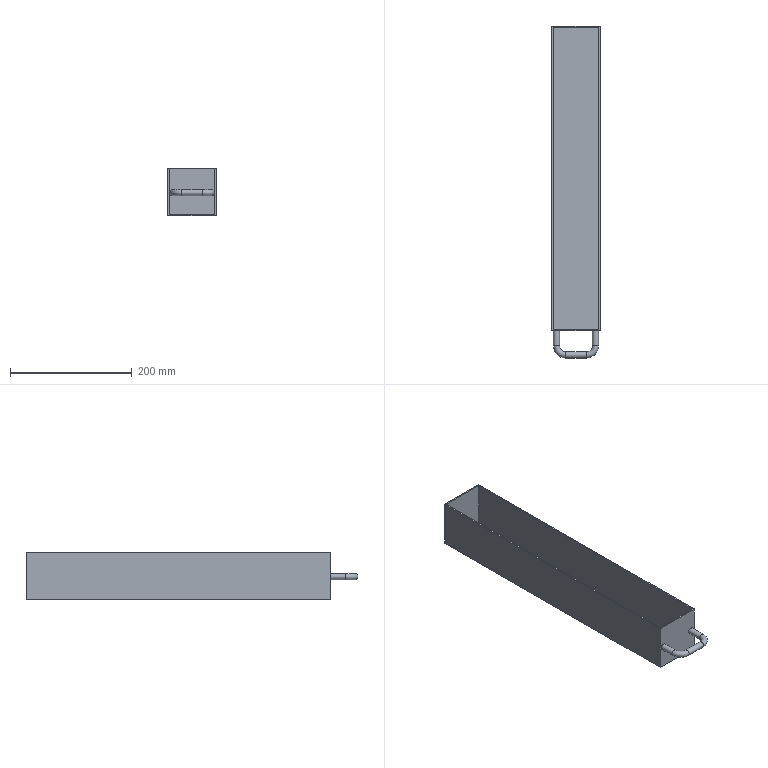Part | NX | features solid 2 | 1 solid | 16 faces | box 79 x 545 x 78 mm | volume 264098 mm3 | plane 11 | cylinder 3 | torus 2 | commonest cylinder face diameters 10 x3
STEP:
#1=CARTESIAN_POINT('',(-464.,-405.,-320.));
#2=VERTEX_POINT('',#1);
#3=CARTESIAN_POINT('',(-385.,-405.,-320.));
#4=VERTEX_POINT('',#3);
#5=CARTESIAN_POINT('',(-910.,-405.,-320.));
#6=DIRECTION('',(1.,0.,0.));
#7=VECTOR('',#6,1000.);
#8=LINE('',#5,#7);
#9=EDGE_CURVE('',#2,#4,#8,.T.);
#10=ORIENTED_EDGE('',*,*,#9,.T.);
#11=CARTESIAN_POINT('',(-385.,-405.,-242.));
#12=VERTEX_POINT('',#11);
#13=CARTESIAN_POINT('',(-385.,-405.,200.));
#14=DIRECTION('',(0.,0.,1.));
#15=VECTOR('',#14,1000.);
#16=LINE('',#13,#15);
#17=EDGE_CURVE('',#12,#4,#16,.F.);
#18=ORIENTED_EDGE('',*,*,#17,.F.);
#19=CARTESIAN_POINT('',(-464.,-405.,-242.));
#20=VERTEX_POINT('',#19);
#21=CARTESIAN_POINT('',(-910.,-405.,-242.));
#22=DIRECTION('',(-1.,0.,0.));
#23=VECTOR('',#22,1000.);
#24=LINE('',#21,#23);
#25=EDGE_CURVE('',#20,#12,#24,.F.);
#26=ORIENTED_EDGE('',*,*,#25,.F.);
#27=CARTESIAN_POINT('',(-464.,-405.,-85.));
#28=DIRECTION('',(0.,0.,1.));
#29=VECTOR('',#28,1000.);
#30=LINE('',#27,#29);
#31=EDGE_CURVE('',#20,#2,#30,.F.);
#32=ORIENTED_EDGE('',*,*,#31,.T.);
#33=EDGE_LOOP('',(#10,#18,#26,#32));
#34=FACE_BOUND('',#33,.T.);
#35=CARTESIAN_POINT('',(-451.5,-405.,-282.));
#36=VERTEX_POINT('',#35);
#37=CARTESIAN_POINT('',(-456.5,-405.,-282.));
#38=DIRECTION('',(0.,1.,0.));
#39=DIRECTION('',(1.,0.,0.));
#40=AXIS2_PLACEMENT_3D('',#37,#38,#39);
#41=CIRCLE('',#40,5.);
#42=EDGE_CURVE('',#36,#36,#41,.T.);
#43=ORIENTED_EDGE('',*,*,#42,.T.);
#44=EDGE_LOOP('',(#43));
#45=FACE_BOUND('',#44,.T.);
#46=CARTESIAN_POINT('',(-392.5,-405.,-287.));
#47=VERTEX_POINT('',#46);
#48=CARTESIAN_POINT('',(-392.5,-405.,-282.));
#49=DIRECTION('',(0.,-1.,0.));
#50=DIRECTION('',(0.,0.,-1.));
#51=AXIS2_PLACEMENT_3D('',#48,#49,#50);
#52=CIRCLE('',#51,5.);
#53=EDGE_CURVE('',#47,#47,#52,.T.);
#54=ORIENTED_EDGE('',*,*,#53,.F.);
#55=EDGE_LOOP('',(#54));
#56=FACE_BOUND('',#55,.T.);
#57=CARTESIAN_POINT('',(-910.,-405.,-85.));
#58=DIRECTION('',(0.,-1.,0.));
#59=DIRECTION('',(0.,0.,-1.));
#60=AXIS2_PLACEMENT_3D('',#57,#58,#59);
#61=PLANE('',#60);
#62=ADVANCED_FACE('',(#34,#45,#56),#61,.T.);
#63=CARTESIAN_POINT('',(-385.,95.,-320.));
#64=VERTEX_POINT('',#63);
#65=CARTESIAN_POINT('',(-385.,-15.,-320.));
#66=DIRECTION('',(0.,-1.,0.));
#67=VECTOR('',#66,1000.);
#68=LINE('',#65,#67);
#69=EDGE_CURVE('',#4,#64,#68,.F.);
#70=ORIENTED_EDGE('',*,*,#69,.T.);
#71=CARTESIAN_POINT('',(-385.,95.,-242.));
#72=VERTEX_POINT('',#71);
#73=CARTESIAN_POINT('',(-385.,95.,-175.));
#74=DIRECTION('',(0.,0.,1.));
#75=VECTOR('',#74,1000.);
#76=LINE('',#73,#75);
#77=EDGE_CURVE('',#72,#64,#76,.F.);
#78=ORIENTED_EDGE('',*,*,#77,.F.);
#79=CARTESIAN_POINT('',(-385.,-15.,-242.));
#80=DIRECTION('',(0.,1.,0.));
#81=VECTOR('',#80,1000.);
#82=LINE('',#79,#81);
#83=EDGE_CURVE('',#12,#72,#82,.T.);
#84=ORIENTED_EDGE('',*,*,#83,.F.);
#85=ORIENTED_EDGE('',*,*,#17,.T.);
#86=EDGE_LOOP('',(#70,#78,#84,#85));
#87=FACE_BOUND('',#86,.T.);
#88=CARTESIAN_POINT('',(-385.,-15.,200.));
#89=DIRECTION('',(-1.,0.,0.));
#90=DIRECTION('',(0.,0.,1.));
#91=AXIS2_PLACEMENT_3D('',#88,#89,#90);
#92=PLANE('',#91);
#93=ADVANCED_FACE('',(#87),#92,.F.);
#94=CARTESIAN_POINT('',(-464.,95.,-320.));
#95=VERTEX_POINT('',#94);
#96=CARTESIAN_POINT('',(-380.,95.,-320.));
#97=DIRECTION('',(-1.,0.,0.));
#98=VECTOR('',#97,1000.);
#99=LINE('',#96,#98);
#100=EDGE_CURVE('',#64,#95,#99,.T.);
#101=ORIENTED_EDGE('',*,*,#100,.T.);
#102=CARTESIAN_POINT('',(-464.,95.,-242.));
#103=VERTEX_POINT('',#102);
#104=CARTESIAN_POINT('',(-464.,95.,200.));
#105=DIRECTION('',(0.,0.,1.));
#106=VECTOR('',#105,1000.);
#107=LINE('',#104,#106);
#108=EDGE_CURVE('',#103,#95,#107,.F.);
#109=ORIENTED_EDGE('',*,*,#108,.F.);
#110=CARTESIAN_POINT('',(-380.,95.,-242.));
#111=DIRECTION('',(1.,0.,0.));
#112=VECTOR('',#111,1000.);
#113=LINE('',#110,#112);
#114=EDGE_CURVE('',#72,#103,#113,.F.);
#115=ORIENTED_EDGE('',*,*,#114,.F.);
#116=ORIENTED_EDGE('',*,*,#77,.T.);
#117=EDGE_LOOP('',(#101,#109,#115,#116));
#118=FACE_BOUND('',#117,.T.);
#119=CARTESIAN_POINT('',(-380.,95.,-175.));
#120=DIRECTION('',(0.,1.,0.));
#121=DIRECTION('',(-1.,0.,0.));
#122=AXIS2_PLACEMENT_3D('',#119,#120,#121);
#123=PLANE('',#122);
#124=ADVANCED_FACE('',(#118),#123,.T.);
#125=CARTESIAN_POINT('',(-464.,580.,-320.));
#126=DIRECTION('',(0.,1.,0.));
#127=VECTOR('',#126,1000.);
#128=LINE('',#125,#127);
#129=EDGE_CURVE('',#95,#2,#128,.F.);
#130=ORIENTED_EDGE('',*,*,#129,.T.);
#131=ORIENTED_EDGE('',*,*,#31,.F.);
#132=CARTESIAN_POINT('',(-464.,580.,-242.));
#133=DIRECTION('',(0.,-1.,0.));
#134=VECTOR('',#133,1000.);
#135=LINE('',#132,#134);
#136=EDGE_CURVE('',#103,#20,#135,.T.);
#137=ORIENTED_EDGE('',*,*,#136,.F.);
#138=ORIENTED_EDGE('',*,*,#108,.T.);
#139=EDGE_LOOP('',(#130,#131,#137,#138));
#140=FACE_BOUND('',#139,.T.);
#141=CARTESIAN_POINT('',(-464.,580.,200.));
#142=DIRECTION('',(1.,0.,0.));
#143=DIRECTION('',(0.,0.,-1.));
#144=AXIS2_PLACEMENT_3D('',#141,#142,#143);
#145=PLANE('',#144);
#146=ADVANCED_FACE('',(#140),#145,.F.);
#147=CARTESIAN_POINT('',(-387.,-403.,-242.));
#148=VERTEX_POINT('',#147);
#149=CARTESIAN_POINT('',(-387.,93.,-242.));
#150=VERTEX_POINT('',#149);
#151=CARTESIAN_POINT('',(-387.,-15.,-242.));
#152=DIRECTION('',(0.,1.,0.));
#153=VECTOR('',#152,1000.);
#154=LINE('',#151,#153);
#155=EDGE_CURVE('',#148,#150,#154,.T.);
#156=ORIENTED_EDGE('',*,*,#155,.F.);
#157=CARTESIAN_POINT('',(-462.,-403.,-242.));
#158=VERTEX_POINT('',#157);
#159=CARTESIAN_POINT('',(-910.,-403.,-242.));
#160=DIRECTION('',(-1.,0.,0.));
#161=VECTOR('',#160,1000.);
#162=LINE('',#159,#161);
#163=EDGE_CURVE('',#158,#148,#162,.F.);
#164=ORIENTED_EDGE('',*,*,#163,.F.);
#165=CARTESIAN_POINT('',(-462.,93.,-242.));
#166=VERTEX_POINT('',#165);
#167=CARTESIAN_POINT('',(-462.,580.,-242.));
#168=DIRECTION('',(0.,-1.,0.));
#169=VECTOR('',#168,1000.);
#170=LINE('',#167,#169);
#171=EDGE_CURVE('',#166,#158,#170,.T.);
#172=ORIENTED_EDGE('',*,*,#171,.F.);
#173=CARTESIAN_POINT('',(-380.,93.,-242.));
#174=DIRECTION('',(1.,0.,0.));
#175=VECTOR('',#174,1000.);
#176=LINE('',#173,#175);
#177=EDGE_CURVE('',#150,#166,#176,.F.);
#178=ORIENTED_EDGE('',*,*,#177,.F.);
#179=EDGE_LOOP('',(#156,#164,#172,#178));
#180=FACE_BOUND('',#179,.T.);
#181=ORIENTED_EDGE('',*,*,#83,.T.);
#182=ORIENTED_EDGE('',*,*,#114,.T.);
#183=ORIENTED_EDGE('',*,*,#136,.T.);
#184=ORIENTED_EDGE('',*,*,#25,.T.);
#185=EDGE_LOOP('',(#181,#182,#183,#184));
#186=FACE_BOUND('',#185,.T.);
#187=CARTESIAN_POINT('',(-385.,580.,-242.));
#188=DIRECTION('',(0.,0.,1.));
#189=DIRECTION('',(1.,0.,0.));
#190=AXIS2_PLACEMENT_3D('',#187,#188,#189);
#191=PLANE('',#190);
#192=ADVANCED_FACE('',(#180,#186),#191,.T.);
#193=ORIENTED_EDGE('',*,*,#69,.F.);
#194=ORIENTED_EDGE('',*,*,#9,.F.);
#195=ORIENTED_EDGE('',*,*,#129,.F.);
#196=ORIENTED_EDGE('',*,*,#100,.F.);
#197=EDGE_LOOP('',(#193,#194,#195,#196));
#198=FACE_BOUND('',#197,.T.);
#199=CARTESIAN_POINT('',(-350.,-70.,-320.));
#200=DIRECTION('',(0.,0.,-1.));
#201=DIRECTION('',(-1.,0.,0.));
#202=AXIS2_PLACEMENT_3D('',#199,#200,#201);
#203=PLANE('',#202);
#204=ADVANCED_FACE('',(#198),#203,.T.);
#205=CARTESIAN_POINT('',(-387.,-403.,-318.));
#206=VERTEX_POINT('',#205);
#207=CARTESIAN_POINT('',(-387.,93.,-318.));
#208=VERTEX_POINT('',#207);
#209=CARTESIAN_POINT('',(-387.,-15.,-318.));
#210=DIRECTION('',(0.,-1.,0.));
#211=VECTOR('',#210,1000.);
#212=LINE('',#209,#211);
#213=EDGE_CURVE('',#206,#208,#212,.F.);
#214=ORIENTED_EDGE('',*,*,#213,.F.);
#215=CARTESIAN_POINT('',(-387.,-403.,200.));
#216=DIRECTION('',(0.,0.,1.));
#217=VECTOR('',#216,1000.);
#218=LINE('',#215,#217);
#219=EDGE_CURVE('',#148,#206,#218,.F.);
#220=ORIENTED_EDGE('',*,*,#219,.F.);
#221=ORIENTED_EDGE('',*,*,#155,.T.);
#222=CARTESIAN_POINT('',(-387.,93.,-175.));
#223=DIRECTION('',(0.,0.,1.));
#224=VECTOR('',#223,1000.);
#225=LINE('',#222,#224);
#226=EDGE_CURVE('',#150,#208,#225,.F.);
#227=ORIENTED_EDGE('',*,*,#226,.T.);
#228=EDGE_LOOP('',(#214,#220,#221,#227));
#229=FACE_BOUND('',#228,.T.);
#230=CARTESIAN_POINT('',(-387.,-15.,200.));
#231=DIRECTION('',(-1.,0.,0.));
#232=DIRECTION('',(0.,0.,1.));
#233=AXIS2_PLACEMENT_3D('',#230,#231,#232);
#234=PLANE('',#233);
#235=ADVANCED_FACE('',(#229),#234,.T.);
#236=CARTESIAN_POINT('',(-462.,93.,-318.));
#237=VERTEX_POINT('',#236);
#238=CARTESIAN_POINT('',(-380.,93.,-318.));
#239=DIRECTION('',(-1.,0.,0.));
#240=VECTOR('',#239,1000.);
#241=LINE('',#238,#240);
#242=EDGE_CURVE('',#208,#237,#241,.T.);
#243=ORIENTED_EDGE('',*,*,#242,.F.);
#244=ORIENTED_EDGE('',*,*,#226,.F.);
#245=ORIENTED_EDGE('',*,*,#177,.T.);
#246=CARTESIAN_POINT('',(-462.,93.,200.));
#247=DIRECTION('',(0.,0.,1.));
#248=VECTOR('',#247,1000.);
#249=LINE('',#246,#248);
#250=EDGE_CURVE('',#166,#237,#249,.F.);
#251=ORIENTED_EDGE('',*,*,#250,.T.);
#252=EDGE_LOOP('',(#243,#244,#245,#251));
#253=FACE_BOUND('',#252,.T.);
#254=CARTESIAN_POINT('',(-380.,93.,-175.));
#255=DIRECTION('',(0.,1.,0.));
#256=DIRECTION('',(-1.,0.,0.));
#257=AXIS2_PLACEMENT_3D('',#254,#255,#256);
#258=PLANE('',#257);
#259=ADVANCED_FACE('',(#253),#258,.F.);
#260=CARTESIAN_POINT('',(-462.,-403.,-318.));
#261=VERTEX_POINT('',#260);
#262=CARTESIAN_POINT('',(-462.,580.,-318.));
#263=DIRECTION('',(0.,1.,0.));
#264=VECTOR('',#263,1000.);
#265=LINE('',#262,#264);
#266=EDGE_CURVE('',#237,#261,#265,.F.);
#267=ORIENTED_EDGE('',*,*,#266,.F.);
#268=ORIENTED_EDGE('',*,*,#250,.F.);
#269=ORIENTED_EDGE('',*,*,#171,.T.);
#270=CARTESIAN_POINT('',(-462.,-403.,-85.));
#271=DIRECTION('',(0.,0.,1.));
#272=VECTOR('',#271,1000.);
#273=LINE('',#270,#272);
#274=EDGE_CURVE('',#158,#261,#273,.F.);
#275=ORIENTED_EDGE('',*,*,#274,.T.);
#276=EDGE_LOOP('',(#267,#268,#269,#275));
#277=FACE_BOUND('',#276,.T.);
#278=CARTESIAN_POINT('',(-462.,580.,200.));
#279=DIRECTION('',(1.,0.,0.));
#280=DIRECTION('',(0.,0.,-1.));
#281=AXIS2_PLACEMENT_3D('',#278,#279,#280);
#282=PLANE('',#281);
#283=ADVANCED_FACE('',(#277),#282,.T.);
#284=CARTESIAN_POINT('',(-910.,-403.,-318.));
#285=DIRECTION('',(1.,0.,0.));
#286=VECTOR('',#285,1000.);
#287=LINE('',#284,#286);
#288=EDGE_CURVE('',#261,#206,#287,.T.);
#289=ORIENTED_EDGE('',*,*,#288,.F.);
#290=ORIENTED_EDGE('',*,*,#274,.F.);
#291=ORIENTED_EDGE('',*,*,#163,.T.);
#292=ORIENTED_EDGE('',*,*,#219,.T.);
#293=EDGE_LOOP('',(#289,#290,#291,#292));
#294=FACE_BOUND('',#293,.T.);
#295=CARTESIAN_POINT('',(-910.,-403.,-85.));
#296=DIRECTION('',(0.,-1.,0.));
#297=DIRECTION('',(0.,0.,-1.));
#298=AXIS2_PLACEMENT_3D('',#295,#296,#297);
#299=PLANE('',#298);
#300=ADVANCED_FACE('',(#294),#299,.F.);
#301=ORIENTED_EDGE('',*,*,#213,.T.);
#302=ORIENTED_EDGE('',*,*,#242,.T.);
#303=ORIENTED_EDGE('',*,*,#266,.T.);
#304=ORIENTED_EDGE('',*,*,#288,.T.);
#305=EDGE_LOOP('',(#301,#302,#303,#304));
#306=FACE_BOUND('',#305,.T.);
#307=CARTESIAN_POINT('',(-350.,-70.,-318.));
#308=DIRECTION('',(0.,0.,-1.));
#309=DIRECTION('',(-1.,0.,0.));
#310=AXIS2_PLACEMENT_3D('',#307,#308,#309);
#311=PLANE('',#310);
#312=ADVANCED_FACE('',(#306),#311,.F.);
#313=CARTESIAN_POINT('',(-407.5,-440.,-282.));
#314=VERTEX_POINT('',#313);
#315=CARTESIAN_POINT('',(-407.5,-445.,-282.));
#316=DIRECTION('',(-1.,0.,0.));
#317=DIRECTION('',(0.,1.,0.));
#318=AXIS2_PLACEMENT_3D('',#315,#316,#317);
#319=CIRCLE('',#318,5.);
#320=EDGE_CURVE('',#314,#314,#319,.T.);
#321=ORIENTED_EDGE('',*,*,#320,.T.);
#322=EDGE_LOOP('',(#321));
#323=FACE_BOUND('',#322,.T.);
#324=CARTESIAN_POINT('',(-441.5,-440.,-282.));
#325=VERTEX_POINT('',#324);
#326=CARTESIAN_POINT('',(-441.5,-445.,-282.));
#327=DIRECTION('',(-1.,0.,0.));
#328=DIRECTION('',(0.,1.,0.));
#329=AXIS2_PLACEMENT_3D('',#326,#327,#328);
#330=CIRCLE('',#329,5.);
#331=EDGE_CURVE('',#325,#325,#330,.T.);
#332=ORIENTED_EDGE('',*,*,#331,.F.);
#333=EDGE_LOOP('',(#332));
#334=FACE_BOUND('',#333,.T.);
#335=CARTESIAN_POINT('',(-457.5,-445.,-282.));
#336=DIRECTION('',(1.,0.,0.));
#337=DIRECTION('',(0.,0.,-1.));
#338=AXIS2_PLACEMENT_3D('',#335,#336,#337);
#339=CYLINDRICAL_SURFACE('',#338,5.);
#340=ADVANCED_FACE('',(#323,#334),#339,.T.);
#341=CARTESIAN_POINT('',(-451.5,-430.,-282.));
#342=VERTEX_POINT('',#341);
#343=CARTESIAN_POINT('',(-456.5,-430.,-282.));
#344=DIRECTION('',(0.,1.,0.));
#345=DIRECTION('',(1.,0.,0.));
#346=AXIS2_PLACEMENT_3D('',#343,#344,#345);
#347=CIRCLE('',#346,5.);
#348=EDGE_CURVE('',#342,#342,#347,.T.);
#349=ORIENTED_EDGE('',*,*,#348,.F.);
#350=EDGE_LOOP('',(#349));
#351=FACE_BOUND('',#350,.T.);
#352=ORIENTED_EDGE('',*,*,#331,.T.);
#353=EDGE_LOOP('',(#352));
#354=FACE_BOUND('',#353,.T.);
#355=CARTESIAN_POINT('',(-441.5,-430.,-282.));
#356=DIRECTION('',(0.,0.,1.));
#357=DIRECTION('',(1.,0.,0.));
#358=AXIS2_PLACEMENT_3D('',#355,#356,#357);
#359=TOROIDAL_SURFACE('',#358,15.,5.);
#360=ADVANCED_FACE('',(#351,#354),#359,.T.);
#361=ORIENTED_EDGE('',*,*,#348,.T.);
#362=EDGE_LOOP('',(#361));
#363=FACE_BOUND('',#362,.T.);
#364=ORIENTED_EDGE('',*,*,#42,.F.);
#365=EDGE_LOOP('',(#364));
#366=FACE_BOUND('',#365,.T.);
#367=CARTESIAN_POINT('',(-456.5,-430.,-282.));
#368=DIRECTION('',(0.,1.,0.));
#369=DIRECTION('',(0.,0.,1.));
#370=AXIS2_PLACEMENT_3D('',#367,#368,#369);
#371=CYLINDRICAL_SURFACE('',#370,5.);
#372=ADVANCED_FACE('',(#363,#366),#371,.T.);
#373=CARTESIAN_POINT('',(-397.5,-430.,-282.));
#374=VERTEX_POINT('',#373);
#375=CARTESIAN_POINT('',(-392.5,-430.,-282.));
#376=DIRECTION('',(0.,-1.,0.));
#377=DIRECTION('',(-1.,0.,0.));
#378=AXIS2_PLACEMENT_3D('',#375,#376,#377);
#379=CIRCLE('',#378,5.);
#380=EDGE_CURVE('',#374,#374,#379,.T.);
#381=ORIENTED_EDGE('',*,*,#380,.F.);
#382=EDGE_LOOP('',(#381));
#383=FACE_BOUND('',#382,.T.);
#384=ORIENTED_EDGE('',*,*,#53,.T.);
#385=EDGE_LOOP('',(#384));
#386=FACE_BOUND('',#385,.T.);
#387=CARTESIAN_POINT('',(-392.5,-430.,-282.));
#388=DIRECTION('',(0.,1.,0.));
#389=DIRECTION('',(0.,0.,1.));
#390=AXIS2_PLACEMENT_3D('',#387,#388,#389);
#391=CYLINDRICAL_SURFACE('',#390,5.);
#392=ADVANCED_FACE('',(#383,#386),#391,.T.);
#393=ORIENTED_EDGE('',*,*,#320,.F.);
#394=EDGE_LOOP('',(#393));
#395=FACE_BOUND('',#394,.T.);
#396=ORIENTED_EDGE('',*,*,#380,.T.);
#397=EDGE_LOOP('',(#396));
#398=FACE_BOUND('',#397,.T.);
#399=CARTESIAN_POINT('',(-407.5,-430.,-282.));
#400=DIRECTION('',(0.,0.,1.));
#401=DIRECTION('',(1.,0.,0.));
#402=AXIS2_PLACEMENT_3D('',#399,#400,#401);
#403=TOROIDAL_SURFACE('',#402,15.,5.);
#404=ADVANCED_FACE('',(#395,#398),#403,.T.);
#405=CLOSED_SHELL('',(#62,#93,#124,#146,#192,#204,#235,#259,#283,#300,#312,#340,#360,#372,#392,#404));
#406=MANIFOLD_SOLID_BREP('',#405);
#407=(LENGTH_UNIT()NAMED_UNIT(*)SI_UNIT(.MILLI.,.METRE.));
#408=UNCERTAINTY_MEASURE_WITH_UNIT(LENGTH_MEASURE(0.00001),#407,'','');
#409=(NAMED_UNIT(*)PLANE_ANGLE_UNIT()SI_UNIT($,.RADIAN.));
#410=(NAMED_UNIT(*)SI_UNIT($,.STERADIAN.)SOLID_ANGLE_UNIT());
#411=(GEOMETRIC_REPRESENTATION_CONTEXT(3)GLOBAL_UNCERTAINTY_ASSIGNED_CONTEXT((#408))GLOBAL_UNIT_ASSIGNED_CONTEXT((#407,#409,#410))REPRESENTATION_CONTEXT('',''));
#412=ADVANCED_BREP_SHAPE_REPRESENTATION('',(#406),#411);